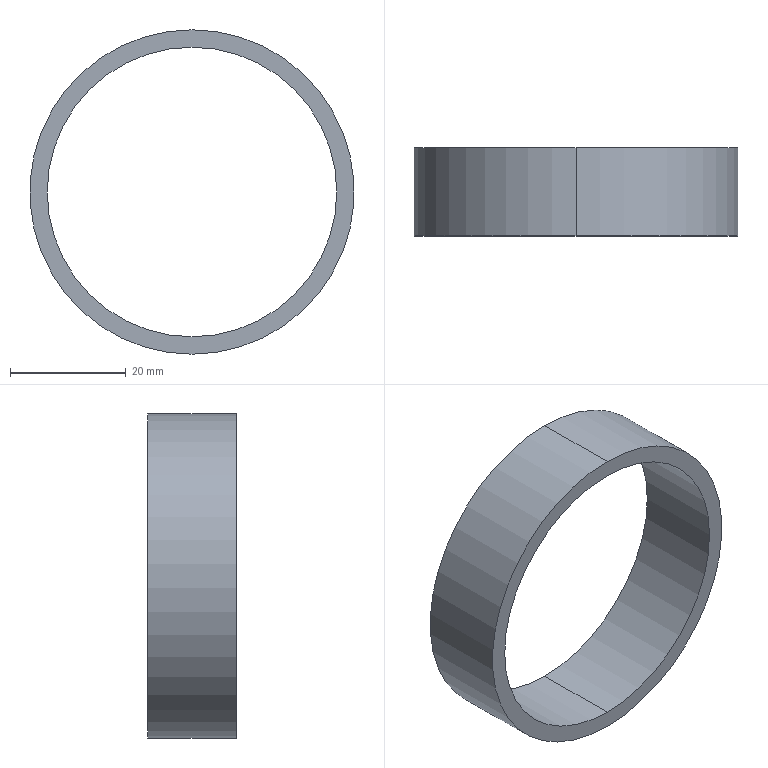Part | STEP file | 0229_209_Color | 1 solid | 6 faces | box 56 x 15.2 x 56 mm | volume 7593 mm3 | cylinder 4 | plane 2 | commonest cylinder face diameters 50 x2 56 x2
STEP:
#1=CARTESIAN_POINT('',(0.,0.,0.));
#2=DIRECTION('',(0.,0.,1.));
#3=DIRECTION('',(1.,0.,0.));
#4=AXIS2_PLACEMENT_3D('',#1,#2,#3);
#5=CARTESIAN_POINT('',(0.,15.2,-28.));
#6=VERTEX_POINT('',#5);
#7=CARTESIAN_POINT('',(0.,15.2,28.));
#8=VERTEX_POINT('',#7);
#9=CARTESIAN_POINT('',(0.,15.2,0.));
#10=DIRECTION('',(0.,-1.,0.));
#11=DIRECTION('',(0.,0.,-1.));
#12=AXIS2_PLACEMENT_3D('',#9,#10,#11);
#13=CIRCLE('',#12,28.);
#14=CARTESIAN_POINT('',(0.,-5.726,0.));
#15=DIRECTION('',(0.,-1.,0.));
#16=DIRECTION('',(0.,0.,-1.));
#17=AXIS2_PLACEMENT_3D('',#14,#15,#16);
#18=CYLINDRICAL_SURFACE('',#17,28.);
#19=CARTESIAN_POINT('',(0.,-20.926));
#20=DIRECTION('',(1.,0.));
#21=VECTOR('',#20,1.);
#22=LINE('',#19,#21);
#23=(GEOMETRIC_REPRESENTATION_CONTEXT(2)PARAMETRIC_REPRESENTATION_CONTEXT()REPRESENTATION_CONTEXT('',''));
#24=DEFINITIONAL_REPRESENTATION('',(#22),#23);
#25=PCURVE('',#18,#24);
#26=CARTESIAN_POINT('',(-25.,15.2,0.));
#27=DIRECTION('',(0.,-1.,0.));
#28=DIRECTION('',(0.,0.,-1.));
#29=AXIS2_PLACEMENT_3D('',#26,#27,#28);
#30=PLANE('',#29);
#31=CARTESIAN_POINT('',(0.,25.));
#32=DIRECTION('',(1.,0.));
#33=AXIS2_PLACEMENT_2D('',#31,#32);
#34=CIRCLE('',#33,28.);
#35=(GEOMETRIC_REPRESENTATION_CONTEXT(2)PARAMETRIC_REPRESENTATION_CONTEXT()REPRESENTATION_CONTEXT('',''));
#36=DEFINITIONAL_REPRESENTATION('',(#34),#35);
#37=PCURVE('',#30,#36);
#38=SURFACE_CURVE('',#13,(#25,#37),.PCURVE_S1.);
#39=EDGE_CURVE('',#6,#8,#38,.T.);
#40=ORIENTED_EDGE('',*,*,#39,.T.);
#41=CARTESIAN_POINT('',(0.,0.,28.));
#42=VERTEX_POINT('',#41);
#43=CARTESIAN_POINT('',(0.,-5.726,28.));
#44=DIRECTION('',(0.,-1.,0.));
#45=VECTOR('',#44,1.);
#46=LINE('',#43,#45);
#47=CARTESIAN_POINT('',(3.142,0.));
#48=DIRECTION('',(0.,1.));
#49=VECTOR('',#48,1.);
#50=LINE('',#47,#49);
#51=(GEOMETRIC_REPRESENTATION_CONTEXT(2)PARAMETRIC_REPRESENTATION_CONTEXT()REPRESENTATION_CONTEXT('',''));
#52=DEFINITIONAL_REPRESENTATION('',(#50),#51);
#53=PCURVE('',#18,#52);
#54=CARTESIAN_POINT('',(0.,-5.726,0.));
#55=DIRECTION('',(0.,-1.,0.));
#56=DIRECTION('',(0.,0.,-1.));
#57=AXIS2_PLACEMENT_3D('',#54,#55,#56);
#58=CYLINDRICAL_SURFACE('',#57,28.);
#59=CARTESIAN_POINT('',(3.142,0.));
#60=DIRECTION('',(0.,1.));
#61=VECTOR('',#60,1.);
#62=LINE('',#59,#61);
#63=(GEOMETRIC_REPRESENTATION_CONTEXT(2)PARAMETRIC_REPRESENTATION_CONTEXT()REPRESENTATION_CONTEXT('',''));
#64=DEFINITIONAL_REPRESENTATION('',(#62),#63);
#65=PCURVE('',#58,#64);
#66=SURFACE_CURVE('',#46,(#53,#65),.PCURVE_S1.);
#67=EDGE_CURVE('',#8,#42,#66,.T.);
#68=ORIENTED_EDGE('',*,*,#67,.T.);
#69=CARTESIAN_POINT('',(0.,0.,-28.));
#70=VERTEX_POINT('',#69);
#71=CARTESIAN_POINT('',(0.,0.,0.));
#72=DIRECTION('',(0.,-1.,0.));
#73=DIRECTION('',(0.,0.,-1.));
#74=AXIS2_PLACEMENT_3D('',#71,#72,#73);
#75=CIRCLE('',#74,28.);
#76=CARTESIAN_POINT('',(0.,-5.726));
#77=DIRECTION('',(1.,0.));
#78=VECTOR('',#77,1.);
#79=LINE('',#76,#78);
#80=(GEOMETRIC_REPRESENTATION_CONTEXT(2)PARAMETRIC_REPRESENTATION_CONTEXT()REPRESENTATION_CONTEXT('',''));
#81=DEFINITIONAL_REPRESENTATION('',(#79),#80);
#82=PCURVE('',#18,#81);
#83=CARTESIAN_POINT('',(-25.,0.,0.));
#84=DIRECTION('',(0.,1.,0.));
#85=DIRECTION('',(0.,0.,1.));
#86=AXIS2_PLACEMENT_3D('',#83,#84,#85);
#87=PLANE('',#86);
#88=CARTESIAN_POINT('',(-28.,25.));
#89=CARTESIAN_POINT('',(-28.,73.497));
#90=CARTESIAN_POINT('',(14.,49.249));
#91=CARTESIAN_POINT('',(56.,25.));
#92=CARTESIAN_POINT('',(14.,0.7513));
#93=CARTESIAN_POINT('',(-28.,-23.497));
#94=CARTESIAN_POINT('',(-28.,25.));
#95=(BOUNDED_CURVE()B_SPLINE_CURVE(2,(#88,#89,#90,#91,#92,#93,#94),.UNSPECIFIED.,.T.,.F.)B_SPLINE_CURVE_WITH_KNOTS((1,2,2,2,2,1),(-2.094,0.,2.094,4.189,6.283,8.378),.UNSPECIFIED.)CURVE()GEOMETRIC_REPRESENTATION_ITEM()RATIONAL_B_SPLINE_CURVE((1.,0.5,1.,0.5,1.,0.5,1.))REPRESENTATION_ITEM(''));
#96=(GEOMETRIC_REPRESENTATION_CONTEXT(2)PARAMETRIC_REPRESENTATION_CONTEXT()REPRESENTATION_CONTEXT('',''));
#97=DEFINITIONAL_REPRESENTATION('',(#95),#96);
#98=PCURVE('',#87,#97);
#99=SURFACE_CURVE('',#75,(#82,#98),.PCURVE_S1.);
#100=EDGE_CURVE('',#70,#42,#99,.T.);
#101=ORIENTED_EDGE('',*,*,#100,.F.);
#102=CARTESIAN_POINT('',(0.,-5.726,-28.));
#103=DIRECTION('',(0.,-1.,0.));
#104=VECTOR('',#103,1.);
#105=LINE('',#102,#104);
#106=CARTESIAN_POINT('',(0.,0.));
#107=DIRECTION('',(0.,1.));
#108=VECTOR('',#107,1.);
#109=LINE('',#106,#108);
#110=(GEOMETRIC_REPRESENTATION_CONTEXT(2)PARAMETRIC_REPRESENTATION_CONTEXT()REPRESENTATION_CONTEXT('',''));
#111=DEFINITIONAL_REPRESENTATION('',(#109),#110);
#112=PCURVE('',#18,#111);
#113=CARTESIAN_POINT('',(6.283,0.));
#114=DIRECTION('',(0.,1.));
#115=VECTOR('',#114,1.);
#116=LINE('',#113,#115);
#117=(GEOMETRIC_REPRESENTATION_CONTEXT(2)PARAMETRIC_REPRESENTATION_CONTEXT()REPRESENTATION_CONTEXT('',''));
#118=DEFINITIONAL_REPRESENTATION('',(#116),#117);
#119=PCURVE('',#58,#118);
#120=SURFACE_CURVE('',#105,(#112,#119),.PCURVE_S1.);
#121=EDGE_CURVE('',#6,#70,#120,.T.);
#122=ORIENTED_EDGE('',*,*,#121,.F.);
#123=EDGE_LOOP('',(#40,#68,#101,#122));
#124=FACE_BOUND('',#123,.T.);
#125=ADVANCED_FACE('',(#124),#18,.T.);
#126=CARTESIAN_POINT('',(0.,15.2,-25.));
#127=VERTEX_POINT('',#126);
#128=CARTESIAN_POINT('',(0.,0.,-25.));
#129=VERTEX_POINT('',#128);
#130=CARTESIAN_POINT('',(0.,-5.726,-25.));
#131=DIRECTION('',(0.,-1.,0.));
#132=VECTOR('',#131,1.);
#133=LINE('',#130,#132);
#134=CARTESIAN_POINT('',(0.,-5.726,0.));
#135=DIRECTION('',(0.,-1.,0.));
#136=DIRECTION('',(0.,0.,-1.));
#137=AXIS2_PLACEMENT_3D('',#134,#135,#136);
#138=CYLINDRICAL_SURFACE('',#137,25.);
#139=CARTESIAN_POINT('',(6.283,0.));
#140=DIRECTION('',(0.,1.));
#141=VECTOR('',#140,1.);
#142=LINE('',#139,#141);
#143=(GEOMETRIC_REPRESENTATION_CONTEXT(2)PARAMETRIC_REPRESENTATION_CONTEXT()REPRESENTATION_CONTEXT('',''));
#144=DEFINITIONAL_REPRESENTATION('',(#142),#143);
#145=PCURVE('',#138,#144);
#146=CARTESIAN_POINT('',(0.,-5.726,0.));
#147=DIRECTION('',(0.,-1.,0.));
#148=DIRECTION('',(0.,0.,-1.));
#149=AXIS2_PLACEMENT_3D('',#146,#147,#148);
#150=CYLINDRICAL_SURFACE('',#149,25.);
#151=CARTESIAN_POINT('',(0.,0.));
#152=DIRECTION('',(0.,1.));
#153=VECTOR('',#152,1.);
#154=LINE('',#151,#153);
#155=(GEOMETRIC_REPRESENTATION_CONTEXT(2)PARAMETRIC_REPRESENTATION_CONTEXT()REPRESENTATION_CONTEXT('',''));
#156=DEFINITIONAL_REPRESENTATION('',(#154),#155);
#157=PCURVE('',#150,#156);
#158=SURFACE_CURVE('',#133,(#145,#157),.PCURVE_S1.);
#159=EDGE_CURVE('',#127,#129,#158,.T.);
#160=ORIENTED_EDGE('',*,*,#159,.T.);
#161=CARTESIAN_POINT('',(0.,0.,25.));
#162=VERTEX_POINT('',#161);
#163=CARTESIAN_POINT('',(0.,0.,0.));
#164=DIRECTION('',(0.,-1.,0.));
#165=DIRECTION('',(0.,0.,-1.));
#166=AXIS2_PLACEMENT_3D('',#163,#164,#165);
#167=CIRCLE('',#166,25.);
#168=CARTESIAN_POINT('',(0.,-5.726));
#169=DIRECTION('',(1.,0.));
#170=VECTOR('',#169,1.);
#171=LINE('',#168,#170);
#172=(GEOMETRIC_REPRESENTATION_CONTEXT(2)PARAMETRIC_REPRESENTATION_CONTEXT()REPRESENTATION_CONTEXT('',''));
#173=DEFINITIONAL_REPRESENTATION('',(#171),#172);
#174=PCURVE('',#138,#173);
#175=CARTESIAN_POINT('',(-25.,25.));
#176=CARTESIAN_POINT('',(-25.,68.301));
#177=CARTESIAN_POINT('',(12.5,46.651));
#178=CARTESIAN_POINT('',(50.,25.));
#179=CARTESIAN_POINT('',(12.5,3.349));
#180=CARTESIAN_POINT('',(-25.,-18.301));
#181=CARTESIAN_POINT('',(-25.,25.));
#182=(BOUNDED_CURVE()B_SPLINE_CURVE(2,(#175,#176,#177,#178,#179,#180,#181),.UNSPECIFIED.,.T.,.F.)B_SPLINE_CURVE_WITH_KNOTS((1,2,2,2,2,1),(-2.094,0.,2.094,4.189,6.283,8.378),.UNSPECIFIED.)CURVE()GEOMETRIC_REPRESENTATION_ITEM()RATIONAL_B_SPLINE_CURVE((1.,0.5,1.,0.5,1.,0.5,1.))REPRESENTATION_ITEM(''));
#183=(GEOMETRIC_REPRESENTATION_CONTEXT(2)PARAMETRIC_REPRESENTATION_CONTEXT()REPRESENTATION_CONTEXT('',''));
#184=DEFINITIONAL_REPRESENTATION('',(#182),#183);
#185=PCURVE('',#87,#184);
#186=SURFACE_CURVE('',#167,(#174,#185),.PCURVE_S1.);
#187=EDGE_CURVE('',#162,#129,#186,.T.);
#188=ORIENTED_EDGE('',*,*,#187,.F.);
#189=CARTESIAN_POINT('',(0.,15.2,25.));
#190=VERTEX_POINT('',#189);
#191=CARTESIAN_POINT('',(0.,-5.726,25.));
#192=DIRECTION('',(0.,-1.,0.));
#193=VECTOR('',#192,1.);
#194=LINE('',#191,#193);
#195=CARTESIAN_POINT('',(3.142,0.));
#196=DIRECTION('',(0.,1.));
#197=VECTOR('',#196,1.);
#198=LINE('',#195,#197);
#199=(GEOMETRIC_REPRESENTATION_CONTEXT(2)PARAMETRIC_REPRESENTATION_CONTEXT()REPRESENTATION_CONTEXT('',''));
#200=DEFINITIONAL_REPRESENTATION('',(#198),#199);
#201=PCURVE('',#138,#200);
#202=CARTESIAN_POINT('',(3.142,0.));
#203=DIRECTION('',(0.,1.));
#204=VECTOR('',#203,1.);
#205=LINE('',#202,#204);
#206=(GEOMETRIC_REPRESENTATION_CONTEXT(2)PARAMETRIC_REPRESENTATION_CONTEXT()REPRESENTATION_CONTEXT('',''));
#207=DEFINITIONAL_REPRESENTATION('',(#205),#206);
#208=PCURVE('',#150,#207);
#209=SURFACE_CURVE('',#194,(#201,#208),.PCURVE_S1.);
#210=EDGE_CURVE('',#190,#162,#209,.T.);
#211=ORIENTED_EDGE('',*,*,#210,.F.);
#212=CARTESIAN_POINT('',(0.,15.2,0.));
#213=DIRECTION('',(0.,-1.,0.));
#214=DIRECTION('',(0.,0.,-1.));
#215=AXIS2_PLACEMENT_3D('',#212,#213,#214);
#216=CIRCLE('',#215,25.);
#217=CARTESIAN_POINT('',(0.,-20.926));
#218=DIRECTION('',(1.,0.));
#219=VECTOR('',#218,1.);
#220=LINE('',#217,#219);
#221=(GEOMETRIC_REPRESENTATION_CONTEXT(2)PARAMETRIC_REPRESENTATION_CONTEXT()REPRESENTATION_CONTEXT('',''));
#222=DEFINITIONAL_REPRESENTATION('',(#220),#221);
#223=PCURVE('',#138,#222);
#224=CARTESIAN_POINT('',(0.,25.));
#225=DIRECTION('',(1.,0.));
#226=AXIS2_PLACEMENT_2D('',#224,#225);
#227=CIRCLE('',#226,25.);
#228=(GEOMETRIC_REPRESENTATION_CONTEXT(2)PARAMETRIC_REPRESENTATION_CONTEXT()REPRESENTATION_CONTEXT('',''));
#229=DEFINITIONAL_REPRESENTATION('',(#227),#228);
#230=PCURVE('',#30,#229);
#231=SURFACE_CURVE('',#216,(#223,#230),.PCURVE_S1.);
#232=EDGE_CURVE('',#190,#127,#231,.T.);
#233=ORIENTED_EDGE('',*,*,#232,.T.);
#234=EDGE_LOOP('',(#160,#188,#211,#233));
#235=FACE_BOUND('',#234,.F.);
#236=ADVANCED_FACE('',(#235),#138,.F.);
#237=CARTESIAN_POINT('',(0.,0.,0.));
#238=DIRECTION('',(0.,-1.,0.));
#239=DIRECTION('',(0.,0.,-1.));
#240=AXIS2_PLACEMENT_3D('',#237,#238,#239);
#241=CIRCLE('',#240,25.);
#242=CARTESIAN_POINT('',(0.,-5.726));
#243=DIRECTION('',(1.,0.));
#244=VECTOR('',#243,1.);
#245=LINE('',#242,#244);
#246=(GEOMETRIC_REPRESENTATION_CONTEXT(2)PARAMETRIC_REPRESENTATION_CONTEXT()REPRESENTATION_CONTEXT('',''));
#247=DEFINITIONAL_REPRESENTATION('',(#245),#246);
#248=PCURVE('',#150,#247);
#249=CARTESIAN_POINT('',(-25.,25.));
#250=CARTESIAN_POINT('',(-25.,68.301));
#251=CARTESIAN_POINT('',(12.5,46.651));
#252=CARTESIAN_POINT('',(50.,25.));
#253=CARTESIAN_POINT('',(12.5,3.349));
#254=CARTESIAN_POINT('',(-25.,-18.301));
#255=CARTESIAN_POINT('',(-25.,25.));
#256=(BOUNDED_CURVE()B_SPLINE_CURVE(2,(#249,#250,#251,#252,#253,#254,#255),.UNSPECIFIED.,.T.,.F.)B_SPLINE_CURVE_WITH_KNOTS((1,2,2,2,2,1),(-2.094,0.,2.094,4.189,6.283,8.378),.UNSPECIFIED.)CURVE()GEOMETRIC_REPRESENTATION_ITEM()RATIONAL_B_SPLINE_CURVE((1.,0.5,1.,0.5,1.,0.5,1.))REPRESENTATION_ITEM(''));
#257=(GEOMETRIC_REPRESENTATION_CONTEXT(2)PARAMETRIC_REPRESENTATION_CONTEXT()REPRESENTATION_CONTEXT('',''));
#258=DEFINITIONAL_REPRESENTATION('',(#256),#257);
#259=PCURVE('',#87,#258);
#260=SURFACE_CURVE('',#241,(#248,#259),.PCURVE_S1.);
#261=EDGE_CURVE('',#129,#162,#260,.T.);
#262=ORIENTED_EDGE('',*,*,#261,.F.);
#263=ORIENTED_EDGE('',*,*,#159,.F.);
#264=CARTESIAN_POINT('',(0.,15.2,0.));
#265=DIRECTION('',(0.,-1.,0.));
#266=DIRECTION('',(0.,0.,-1.));
#267=AXIS2_PLACEMENT_3D('',#264,#265,#266);
#268=CIRCLE('',#267,25.);
#269=CARTESIAN_POINT('',(0.,-20.926));
#270=DIRECTION('',(1.,0.));
#271=VECTOR('',#270,1.);
#272=LINE('',#269,#271);
#273=(GEOMETRIC_REPRESENTATION_CONTEXT(2)PARAMETRIC_REPRESENTATION_CONTEXT()REPRESENTATION_CONTEXT('',''));
#274=DEFINITIONAL_REPRESENTATION('',(#272),#273);
#275=PCURVE('',#150,#274);
#276=CARTESIAN_POINT('',(0.,25.));
#277=DIRECTION('',(1.,0.));
#278=AXIS2_PLACEMENT_2D('',#276,#277);
#279=CIRCLE('',#278,25.);
#280=(GEOMETRIC_REPRESENTATION_CONTEXT(2)PARAMETRIC_REPRESENTATION_CONTEXT()REPRESENTATION_CONTEXT('',''));
#281=DEFINITIONAL_REPRESENTATION('',(#279),#280);
#282=PCURVE('',#30,#281);
#283=SURFACE_CURVE('',#268,(#275,#282),.PCURVE_S1.);
#284=EDGE_CURVE('',#127,#190,#283,.T.);
#285=ORIENTED_EDGE('',*,*,#284,.T.);
#286=ORIENTED_EDGE('',*,*,#210,.T.);
#287=EDGE_LOOP('',(#262,#263,#285,#286));
#288=FACE_BOUND('',#287,.F.);
#289=ADVANCED_FACE('',(#288),#150,.F.);
#290=ORIENTED_EDGE('',*,*,#39,.F.);
#291=CARTESIAN_POINT('',(0.,15.2,0.));
#292=DIRECTION('',(0.,-1.,0.));
#293=DIRECTION('',(0.,0.,-1.));
#294=AXIS2_PLACEMENT_3D('',#291,#292,#293);
#295=CIRCLE('',#294,28.);
#296=CARTESIAN_POINT('',(0.,25.));
#297=DIRECTION('',(1.,0.));
#298=AXIS2_PLACEMENT_2D('',#296,#297);
#299=CIRCLE('',#298,28.);
#300=(GEOMETRIC_REPRESENTATION_CONTEXT(2)PARAMETRIC_REPRESENTATION_CONTEXT()REPRESENTATION_CONTEXT('',''));
#301=DEFINITIONAL_REPRESENTATION('',(#299),#300);
#302=PCURVE('',#30,#301);
#303=CARTESIAN_POINT('',(0.,-20.926));
#304=DIRECTION('',(1.,0.));
#305=VECTOR('',#304,1.);
#306=LINE('',#303,#305);
#307=(GEOMETRIC_REPRESENTATION_CONTEXT(2)PARAMETRIC_REPRESENTATION_CONTEXT()REPRESENTATION_CONTEXT('',''));
#308=DEFINITIONAL_REPRESENTATION('',(#306),#307);
#309=PCURVE('',#58,#308);
#310=SURFACE_CURVE('',#295,(#302,#309),.PCURVE_S1.);
#311=EDGE_CURVE('',#8,#6,#310,.T.);
#312=ORIENTED_EDGE('',*,*,#311,.F.);
#313=EDGE_LOOP('',(#290,#312));
#314=FACE_BOUND('',#313,.T.);
#315=ORIENTED_EDGE('',*,*,#284,.T.);
#316=ORIENTED_EDGE('',*,*,#232,.T.);
#317=EDGE_LOOP('',(#315,#316));
#318=FACE_BOUND('',#317,.T.);
#319=ADVANCED_FACE('',(#314,#318),#30,.F.);
#320=ORIENTED_EDGE('',*,*,#67,.F.);
#321=ORIENTED_EDGE('',*,*,#311,.T.);
#322=ORIENTED_EDGE('',*,*,#121,.T.);
#323=CARTESIAN_POINT('',(0.,0.,0.));
#324=DIRECTION('',(0.,-1.,0.));
#325=DIRECTION('',(0.,0.,-1.));
#326=AXIS2_PLACEMENT_3D('',#323,#324,#325);
#327=CIRCLE('',#326,28.);
#328=CARTESIAN_POINT('',(0.,-5.726));
#329=DIRECTION('',(1.,0.));
#330=VECTOR('',#329,1.);
#331=LINE('',#328,#330);
#332=(GEOMETRIC_REPRESENTATION_CONTEXT(2)PARAMETRIC_REPRESENTATION_CONTEXT()REPRESENTATION_CONTEXT('',''));
#333=DEFINITIONAL_REPRESENTATION('',(#331),#332);
#334=PCURVE('',#58,#333);
#335=CARTESIAN_POINT('',(-28.,25.));
#336=CARTESIAN_POINT('',(-28.,73.497));
#337=CARTESIAN_POINT('',(14.,49.249));
#338=CARTESIAN_POINT('',(56.,25.));
#339=CARTESIAN_POINT('',(14.,0.7513));
#340=CARTESIAN_POINT('',(-28.,-23.497));
#341=CARTESIAN_POINT('',(-28.,25.));
#342=(BOUNDED_CURVE()B_SPLINE_CURVE(2,(#335,#336,#337,#338,#339,#340,#341),.UNSPECIFIED.,.T.,.F.)B_SPLINE_CURVE_WITH_KNOTS((1,2,2,2,2,1),(-2.094,0.,2.094,4.189,6.283,8.378),.UNSPECIFIED.)CURVE()GEOMETRIC_REPRESENTATION_ITEM()RATIONAL_B_SPLINE_CURVE((1.,0.5,1.,0.5,1.,0.5,1.))REPRESENTATION_ITEM(''));
#343=(GEOMETRIC_REPRESENTATION_CONTEXT(2)PARAMETRIC_REPRESENTATION_CONTEXT()REPRESENTATION_CONTEXT('',''));
#344=DEFINITIONAL_REPRESENTATION('',(#342),#343);
#345=PCURVE('',#87,#344);
#346=SURFACE_CURVE('',#327,(#334,#345),.PCURVE_S1.);
#347=EDGE_CURVE('',#42,#70,#346,.T.);
#348=ORIENTED_EDGE('',*,*,#347,.F.);
#349=EDGE_LOOP('',(#320,#321,#322,#348));
#350=FACE_BOUND('',#349,.T.);
#351=ADVANCED_FACE('',(#350),#58,.T.);
#352=ORIENTED_EDGE('',*,*,#261,.F.);
#353=ORIENTED_EDGE('',*,*,#187,.F.);
#354=EDGE_LOOP('',(#352,#353));
#355=FACE_BOUND('',#354,.T.);
#356=ORIENTED_EDGE('',*,*,#100,.T.);
#357=ORIENTED_EDGE('',*,*,#347,.T.);
#358=EDGE_LOOP('',(#356,#357));
#359=FACE_BOUND('',#358,.T.);
#360=ADVANCED_FACE('',(#355,#359),#87,.F.);
#361=CLOSED_SHELL('',(#125,#236,#289,#319,#351,#360));
#362=MANIFOLD_SOLID_BREP('',#361);
#363=(LENGTH_UNIT()NAMED_UNIT(*)SI_UNIT(.MILLI.,.METRE.));
#364=UNCERTAINTY_MEASURE_WITH_UNIT(LENGTH_MEASURE(0.0000001),#363,'','');
#365=(NAMED_UNIT(*)PLANE_ANGLE_UNIT()SI_UNIT($,.RADIAN.));
#366=(NAMED_UNIT(*)SI_UNIT($,.STERADIAN.)SOLID_ANGLE_UNIT());
#367=(GEOMETRIC_REPRESENTATION_CONTEXT(3)GLOBAL_UNCERTAINTY_ASSIGNED_CONTEXT((#364))GLOBAL_UNIT_ASSIGNED_CONTEXT((#363,#365,#366))REPRESENTATION_CONTEXT('',''));
#368=ADVANCED_BREP_SHAPE_REPRESENTATION('',(#4,#362),#367);